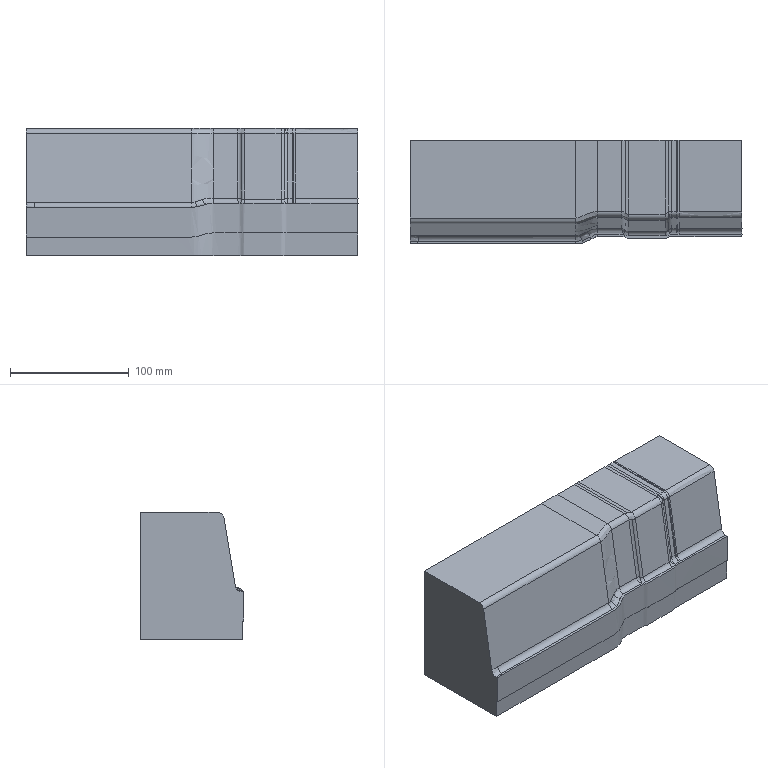Part | NX | features solid 2 | 1 solid | 73 faces | box 280 x 87.161 x 107.138 mm | volume 2279112 mm3 | spline 30 | plane 20 | cylinder 20 | cone 3 | commonest cylinder face diameters 10 x9 8 x5 12 x3 20 x2 14 x1